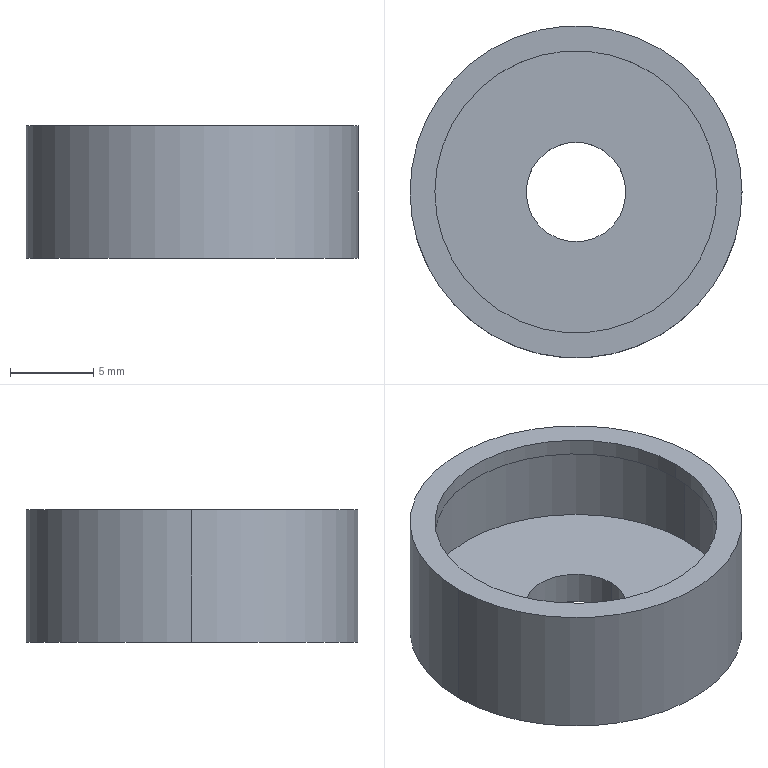Part | SolidWorks | features ICE 3, Extrusion 1 | 1 solid | 12 faces | box 20 x 20 x 8 mm | volume 885.733 mm3 | cylinder 8 | plane 4 | commonest cylinder face diameters 6 x2 17 x2 18.5 x2 20 x2
STEP:
#1=CARTESIAN_POINT('',(-9.25,0.,7.));
#2=VERTEX_POINT('',#1);
#3=CARTESIAN_POINT('',(9.25,0.,7.));
#4=VERTEX_POINT('',#3);
#5=CARTESIAN_POINT('',(0.,0.,7.));
#6=DIRECTION('',(0.,0.,1.));
#7=DIRECTION('',(1.,0.,0.));
#8=AXIS2_PLACEMENT_3D('',#5,#6,#7);
#9=CIRCLE('',#8,9.25);
#10=EDGE_CURVE('',#2,#4,#9,.T.);
#11=ORIENTED_EDGE('',*,*,#10,.T.);
#12=CARTESIAN_POINT('',(9.25,0.,2.));
#13=VERTEX_POINT('',#12);
#14=CARTESIAN_POINT('',(9.25,0.,7.));
#15=DIRECTION('',(0.,0.,-1.));
#16=VECTOR('',#15,1000.);
#17=LINE('',#14,#16);
#18=EDGE_CURVE('',#4,#13,#17,.T.);
#19=ORIENTED_EDGE('',*,*,#18,.T.);
#20=CARTESIAN_POINT('',(-9.25,0.,2.));
#21=VERTEX_POINT('',#20);
#22=CARTESIAN_POINT('',(0.,0.,2.));
#23=DIRECTION('',(0.,0.,1.));
#24=DIRECTION('',(1.,0.,0.));
#25=AXIS2_PLACEMENT_3D('',#22,#23,#24);
#26=CIRCLE('',#25,9.25);
#27=EDGE_CURVE('',#21,#13,#26,.T.);
#28=ORIENTED_EDGE('',*,*,#27,.F.);
#29=CARTESIAN_POINT('',(-9.25,0.,7.));
#30=DIRECTION('',(0.,0.,-1.));
#31=VECTOR('',#30,1000.);
#32=LINE('',#29,#31);
#33=EDGE_CURVE('',#2,#21,#32,.T.);
#34=ORIENTED_EDGE('',*,*,#33,.F.);
#35=EDGE_LOOP('',(#11,#19,#28,#34));
#36=FACE_OUTER_BOUND('',#35,.T.);
#37=CARTESIAN_POINT('',(0.,0.,7.));
#38=DIRECTION('',(0.,0.,-1.));
#39=DIRECTION('',(-1.,0.,0.));
#40=AXIS2_PLACEMENT_3D('',#37,#38,#39);
#41=CYLINDRICAL_SURFACE('',#40,9.25);
#42=ADVANCED_FACE('',(#36),#41,.F.);
#43=CARTESIAN_POINT('',(-3.,0.,0.));
#44=VERTEX_POINT('',#43);
#45=CARTESIAN_POINT('',(3.,0.,0.));
#46=VERTEX_POINT('',#45);
#47=CARTESIAN_POINT('',(0.,0.,0.));
#48=DIRECTION('',(0.,0.,1.));
#49=DIRECTION('',(1.,0.,0.));
#50=AXIS2_PLACEMENT_3D('',#47,#48,#49);
#51=CIRCLE('',#50,3.);
#52=EDGE_CURVE('',#44,#46,#51,.T.);
#53=ORIENTED_EDGE('',*,*,#52,.F.);
#54=CARTESIAN_POINT('',(-3.,0.,2.));
#55=VERTEX_POINT('',#54);
#56=CARTESIAN_POINT('',(-3.,0.,0.));
#57=DIRECTION('',(0.,0.,1.));
#58=VECTOR('',#57,1000.);
#59=LINE('',#56,#58);
#60=EDGE_CURVE('',#44,#55,#59,.T.);
#61=ORIENTED_EDGE('',*,*,#60,.T.);
#62=CARTESIAN_POINT('',(3.,0.,2.));
#63=VERTEX_POINT('',#62);
#64=CARTESIAN_POINT('',(0.,0.,2.));
#65=DIRECTION('',(0.,0.,1.));
#66=DIRECTION('',(1.,0.,0.));
#67=AXIS2_PLACEMENT_3D('',#64,#65,#66);
#68=CIRCLE('',#67,3.);
#69=EDGE_CURVE('',#55,#63,#68,.T.);
#70=ORIENTED_EDGE('',*,*,#69,.T.);
#71=CARTESIAN_POINT('',(3.,0.,0.));
#72=DIRECTION('',(0.,0.,1.));
#73=VECTOR('',#72,1000.);
#74=LINE('',#71,#73);
#75=EDGE_CURVE('',#46,#63,#74,.T.);
#76=ORIENTED_EDGE('',*,*,#75,.F.);
#77=EDGE_LOOP('',(#53,#61,#70,#76));
#78=FACE_OUTER_BOUND('',#77,.T.);
#79=CARTESIAN_POINT('',(0.,0.,0.));
#80=DIRECTION('',(0.,0.,1.));
#81=DIRECTION('',(1.,0.,0.));
#82=AXIS2_PLACEMENT_3D('',#79,#80,#81);
#83=CYLINDRICAL_SURFACE('',#82,3.);
#84=ADVANCED_FACE('',(#78),#83,.F.);
#85=CARTESIAN_POINT('',(8.5,0.,7.));
#86=VERTEX_POINT('',#85);
#87=CARTESIAN_POINT('',(-8.5,0.,7.));
#88=VERTEX_POINT('',#87);
#89=CARTESIAN_POINT('',(0.,0.,7.));
#90=DIRECTION('',(0.,0.,-1.));
#91=DIRECTION('',(1.,0.,0.));
#92=AXIS2_PLACEMENT_3D('',#89,#90,#91);
#93=CIRCLE('',#92,8.5);
#94=EDGE_CURVE('',#86,#88,#93,.T.);
#95=ORIENTED_EDGE('',*,*,#94,.T.);
#96=CARTESIAN_POINT('',(-8.5,0.,8.));
#97=VERTEX_POINT('',#96);
#98=CARTESIAN_POINT('',(-8.5,0.,2.));
#99=DIRECTION('',(0.,0.,1.));
#100=VECTOR('',#99,1000.);
#101=LINE('',#98,#100);
#102=EDGE_CURVE('',#88,#97,#101,.T.);
#103=ORIENTED_EDGE('',*,*,#102,.T.);
#104=CARTESIAN_POINT('',(8.5,0.,8.));
#105=VERTEX_POINT('',#104);
#106=CARTESIAN_POINT('',(0.,0.,8.));
#107=DIRECTION('',(0.,0.,1.));
#108=DIRECTION('',(1.,0.,0.));
#109=AXIS2_PLACEMENT_3D('',#106,#107,#108);
#110=CIRCLE('',#109,8.5);
#111=EDGE_CURVE('',#97,#105,#110,.T.);
#112=ORIENTED_EDGE('',*,*,#111,.T.);
#113=CARTESIAN_POINT('',(8.5,0.,2.));
#114=DIRECTION('',(0.,0.,1.));
#115=VECTOR('',#114,1000.);
#116=LINE('',#113,#115);
#117=EDGE_CURVE('',#86,#105,#116,.T.);
#118=ORIENTED_EDGE('',*,*,#117,.F.);
#119=EDGE_LOOP('',(#95,#103,#112,#118));
#120=FACE_OUTER_BOUND('',#119,.T.);
#121=CARTESIAN_POINT('',(0.,0.,2.));
#122=DIRECTION('',(0.,0.,1.));
#123=DIRECTION('',(1.,0.,0.));
#124=AXIS2_PLACEMENT_3D('',#121,#122,#123);
#125=CYLINDRICAL_SURFACE('',#124,8.5);
#126=ADVANCED_FACE('',(#120),#125,.F.);
#127=CARTESIAN_POINT('',(10.,0.,8.));
#128=VERTEX_POINT('',#127);
#129=CARTESIAN_POINT('',(-10.,0.,8.));
#130=VERTEX_POINT('',#129);
#131=CARTESIAN_POINT('',(0.,0.,8.));
#132=DIRECTION('',(0.,0.,1.));
#133=DIRECTION('',(1.,0.,0.));
#134=AXIS2_PLACEMENT_3D('',#131,#132,#133);
#135=CIRCLE('',#134,10.);
#136=EDGE_CURVE('',#128,#130,#135,.T.);
#137=ORIENTED_EDGE('',*,*,#136,.F.);
#138=CARTESIAN_POINT('',(10.,0.,0.));
#139=VERTEX_POINT('',#138);
#140=CARTESIAN_POINT('',(10.,0.,8.));
#141=DIRECTION('',(0.,0.,-1.));
#142=VECTOR('',#141,1000.);
#143=LINE('',#140,#142);
#144=EDGE_CURVE('',#128,#139,#143,.T.);
#145=ORIENTED_EDGE('',*,*,#144,.T.);
#146=CARTESIAN_POINT('',(-10.,0.,0.));
#147=VERTEX_POINT('',#146);
#148=CARTESIAN_POINT('',(0.,0.,0.));
#149=DIRECTION('',(0.,0.,1.));
#150=DIRECTION('',(1.,0.,0.));
#151=AXIS2_PLACEMENT_3D('',#148,#149,#150);
#152=CIRCLE('',#151,10.);
#153=EDGE_CURVE('',#139,#147,#152,.T.);
#154=ORIENTED_EDGE('',*,*,#153,.T.);
#155=CARTESIAN_POINT('',(-10.,0.,8.));
#156=DIRECTION('',(0.,0.,-1.));
#157=VECTOR('',#156,1000.);
#158=LINE('',#155,#157);
#159=EDGE_CURVE('',#130,#147,#158,.T.);
#160=ORIENTED_EDGE('',*,*,#159,.F.);
#161=EDGE_LOOP('',(#137,#145,#154,#160));
#162=FACE_OUTER_BOUND('',#161,.T.);
#163=CARTESIAN_POINT('',(0.,0.,8.));
#164=DIRECTION('',(0.,0.,-1.));
#165=DIRECTION('',(-1.,0.,0.));
#166=AXIS2_PLACEMENT_3D('',#163,#164,#165);
#167=CYLINDRICAL_SURFACE('',#166,10.);
#168=ADVANCED_FACE('',(#162),#167,.T.);
#169=ORIENTED_EDGE('',*,*,#144,.F.);
#170=CARTESIAN_POINT('',(0.,0.,8.));
#171=DIRECTION('',(0.,0.,1.));
#172=DIRECTION('',(1.,0.,0.));
#173=AXIS2_PLACEMENT_3D('',#170,#171,#172);
#174=CIRCLE('',#173,10.);
#175=EDGE_CURVE('',#130,#128,#174,.T.);
#176=ORIENTED_EDGE('',*,*,#175,.F.);
#177=ORIENTED_EDGE('',*,*,#159,.T.);
#178=CARTESIAN_POINT('',(0.,0.,0.));
#179=DIRECTION('',(0.,0.,1.));
#180=DIRECTION('',(1.,0.,0.));
#181=AXIS2_PLACEMENT_3D('',#178,#179,#180);
#182=CIRCLE('',#181,10.);
#183=EDGE_CURVE('',#147,#139,#182,.T.);
#184=ORIENTED_EDGE('',*,*,#183,.T.);
#185=EDGE_LOOP('',(#169,#176,#177,#184));
#186=FACE_OUTER_BOUND('',#185,.T.);
#187=CARTESIAN_POINT('',(0.,0.,8.));
#188=DIRECTION('',(0.,0.,-1.));
#189=DIRECTION('',(-1.,0.,0.));
#190=AXIS2_PLACEMENT_3D('',#187,#188,#189);
#191=CYLINDRICAL_SURFACE('',#190,10.);
#192=ADVANCED_FACE('',(#186),#191,.T.);
#193=CARTESIAN_POINT('',(0.,0.,8.));
#194=DIRECTION('',(0.,0.,1.));
#195=DIRECTION('',(1.,0.,0.));
#196=AXIS2_PLACEMENT_3D('',#193,#194,#195);
#197=CIRCLE('',#196,8.5);
#198=EDGE_CURVE('',#105,#97,#197,.T.);
#199=ORIENTED_EDGE('',*,*,#198,.F.);
#200=ORIENTED_EDGE('',*,*,#111,.F.);
#201=EDGE_LOOP('',(#199,#200));
#202=FACE_BOUND('',#201,.T.);
#203=ORIENTED_EDGE('',*,*,#175,.T.);
#204=ORIENTED_EDGE('',*,*,#136,.T.);
#205=EDGE_LOOP('',(#203,#204));
#206=FACE_OUTER_BOUND('',#205,.T.);
#207=CARTESIAN_POINT('',(0.,0.,8.));
#208=DIRECTION('',(0.,0.,1.));
#209=DIRECTION('',(1.,0.,0.));
#210=AXIS2_PLACEMENT_3D('',#207,#208,#209);
#211=PLANE('',#210);
#212=ADVANCED_FACE('',(#202,#206),#211,.T.);
#213=CARTESIAN_POINT('',(0.,0.,0.));
#214=DIRECTION('',(0.,0.,1.));
#215=DIRECTION('',(1.,0.,0.));
#216=AXIS2_PLACEMENT_3D('',#213,#214,#215);
#217=CIRCLE('',#216,3.);
#218=EDGE_CURVE('',#46,#44,#217,.T.);
#219=ORIENTED_EDGE('',*,*,#218,.T.);
#220=ORIENTED_EDGE('',*,*,#52,.T.);
#221=EDGE_LOOP('',(#219,#220));
#222=FACE_BOUND('',#221,.T.);
#223=ORIENTED_EDGE('',*,*,#183,.F.);
#224=ORIENTED_EDGE('',*,*,#153,.F.);
#225=EDGE_LOOP('',(#223,#224));
#226=FACE_OUTER_BOUND('',#225,.T.);
#227=CARTESIAN_POINT('',(0.,0.,0.));
#228=DIRECTION('',(0.,0.,1.));
#229=DIRECTION('',(1.,0.,0.));
#230=AXIS2_PLACEMENT_3D('',#227,#228,#229);
#231=PLANE('',#230);
#232=ADVANCED_FACE('',(#222,#226),#231,.F.);
#233=ORIENTED_EDGE('',*,*,#102,.F.);
#234=CARTESIAN_POINT('',(0.,0.,7.));
#235=DIRECTION('',(0.,0.,-1.));
#236=DIRECTION('',(1.,0.,0.));
#237=AXIS2_PLACEMENT_3D('',#234,#235,#236);
#238=CIRCLE('',#237,8.5);
#239=EDGE_CURVE('',#88,#86,#238,.T.);
#240=ORIENTED_EDGE('',*,*,#239,.T.);
#241=ORIENTED_EDGE('',*,*,#117,.T.);
#242=ORIENTED_EDGE('',*,*,#198,.T.);
#243=EDGE_LOOP('',(#233,#240,#241,#242));
#244=FACE_OUTER_BOUND('',#243,.T.);
#245=CARTESIAN_POINT('',(0.,0.,2.));
#246=DIRECTION('',(0.,0.,1.));
#247=DIRECTION('',(1.,0.,0.));
#248=AXIS2_PLACEMENT_3D('',#245,#246,#247);
#249=CYLINDRICAL_SURFACE('',#248,8.5);
#250=ADVANCED_FACE('',(#244),#249,.F.);
#251=CARTESIAN_POINT('',(0.,0.,2.));
#252=DIRECTION('',(0.,0.,1.));
#253=DIRECTION('',(1.,0.,0.));
#254=AXIS2_PLACEMENT_3D('',#251,#252,#253);
#255=CIRCLE('',#254,3.);
#256=EDGE_CURVE('',#63,#55,#255,.T.);
#257=ORIENTED_EDGE('',*,*,#256,.F.);
#258=ORIENTED_EDGE('',*,*,#69,.F.);
#259=EDGE_LOOP('',(#257,#258));
#260=FACE_BOUND('',#259,.T.);
#261=ORIENTED_EDGE('',*,*,#27,.T.);
#262=CARTESIAN_POINT('',(0.,0.,2.));
#263=DIRECTION('',(0.,0.,1.));
#264=DIRECTION('',(1.,0.,0.));
#265=AXIS2_PLACEMENT_3D('',#262,#263,#264);
#266=CIRCLE('',#265,9.25);
#267=EDGE_CURVE('',#13,#21,#266,.T.);
#268=ORIENTED_EDGE('',*,*,#267,.T.);
#269=EDGE_LOOP('',(#261,#268));
#270=FACE_OUTER_BOUND('',#269,.T.);
#271=CARTESIAN_POINT('',(0.,0.,2.));
#272=DIRECTION('',(0.,0.,1.));
#273=DIRECTION('',(1.,0.,0.));
#274=AXIS2_PLACEMENT_3D('',#271,#272,#273);
#275=PLANE('',#274);
#276=ADVANCED_FACE('',(#260,#270),#275,.T.);
#277=ORIENTED_EDGE('',*,*,#60,.F.);
#278=ORIENTED_EDGE('',*,*,#218,.F.);
#279=ORIENTED_EDGE('',*,*,#75,.T.);
#280=ORIENTED_EDGE('',*,*,#256,.T.);
#281=EDGE_LOOP('',(#277,#278,#279,#280));
#282=FACE_OUTER_BOUND('',#281,.T.);
#283=CARTESIAN_POINT('',(0.,0.,0.));
#284=DIRECTION('',(0.,0.,1.));
#285=DIRECTION('',(1.,0.,0.));
#286=AXIS2_PLACEMENT_3D('',#283,#284,#285);
#287=CYLINDRICAL_SURFACE('',#286,3.);
#288=ADVANCED_FACE('',(#282),#287,.F.);
#289=ORIENTED_EDGE('',*,*,#10,.F.);
#290=CARTESIAN_POINT('',(0.,0.,7.));
#291=DIRECTION('',(0.,0.,1.));
#292=DIRECTION('',(1.,0.,0.));
#293=AXIS2_PLACEMENT_3D('',#290,#291,#292);
#294=CIRCLE('',#293,9.25);
#295=EDGE_CURVE('',#4,#2,#294,.T.);
#296=ORIENTED_EDGE('',*,*,#295,.F.);
#297=EDGE_LOOP('',(#289,#296));
#298=FACE_OUTER_BOUND('',#297,.T.);
#299=ORIENTED_EDGE('',*,*,#94,.F.);
#300=ORIENTED_EDGE('',*,*,#239,.F.);
#301=EDGE_LOOP('',(#299,#300));
#302=FACE_BOUND('',#301,.T.);
#303=CARTESIAN_POINT('',(0.,0.,7.));
#304=DIRECTION('',(0.,0.,1.));
#305=DIRECTION('',(1.,0.,0.));
#306=AXIS2_PLACEMENT_3D('',#303,#304,#305);
#307=PLANE('',#306);
#308=ADVANCED_FACE('',(#298,#302),#307,.F.);
#309=ORIENTED_EDGE('',*,*,#18,.F.);
#310=ORIENTED_EDGE('',*,*,#295,.T.);
#311=ORIENTED_EDGE('',*,*,#33,.T.);
#312=ORIENTED_EDGE('',*,*,#267,.F.);
#313=EDGE_LOOP('',(#309,#310,#311,#312));
#314=FACE_OUTER_BOUND('',#313,.T.);
#315=CARTESIAN_POINT('',(0.,0.,7.));
#316=DIRECTION('',(0.,0.,-1.));
#317=DIRECTION('',(-1.,0.,0.));
#318=AXIS2_PLACEMENT_3D('',#315,#316,#317);
#319=CYLINDRICAL_SURFACE('',#318,9.25);
#320=ADVANCED_FACE('',(#314),#319,.F.);
#321=CLOSED_SHELL('',(#42,#84,#126,#168,#192,#212,#232,#250,#276,#288,#308,#320));
#322=MANIFOLD_SOLID_BREP('',#321);
#323=CARTESIAN_POINT('',(0.,0.,0.));
#324=DIRECTION('',(0.,0.,1.));
#325=DIRECTION('',(1.,0.,0.));
#326=AXIS2_PLACEMENT_3D('',#323,#324,#325);
#327=(LENGTH_UNIT()NAMED_UNIT(*)SI_UNIT(.MILLI.,.METRE.));
#328=UNCERTAINTY_MEASURE_WITH_UNIT(LENGTH_MEASURE(0.00001),#327,'','');
#329=(NAMED_UNIT(*)PLANE_ANGLE_UNIT()SI_UNIT($,.RADIAN.));
#330=(NAMED_UNIT(*)SI_UNIT($,.STERADIAN.)SOLID_ANGLE_UNIT());
#331=(GEOMETRIC_REPRESENTATION_CONTEXT(3)GLOBAL_UNCERTAINTY_ASSIGNED_CONTEXT((#328))GLOBAL_UNIT_ASSIGNED_CONTEXT((#327,#329,#330))REPRESENTATION_CONTEXT('',''));
#332=ADVANCED_BREP_SHAPE_REPRESENTATION('',(#322,#326),#331);